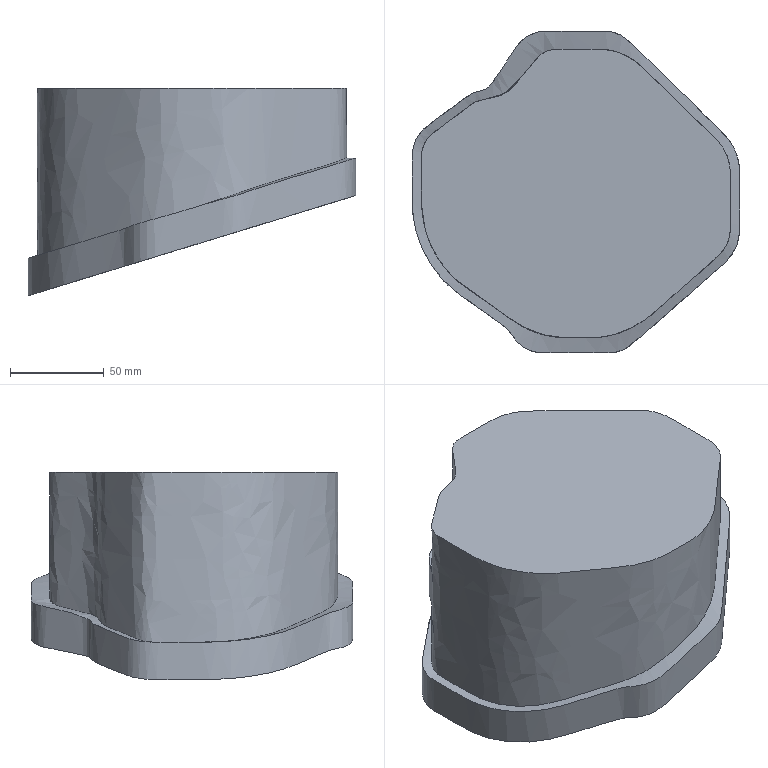Part | NX | features solid 2 | 1 solid | 27 faces | box 175.076 x 171.91 x 110.75 mm | volume 1165177 mm3 | spline 15 | plane 7 | cylinder 5 | commonest cylinder face diameters 30 x3 25 x2